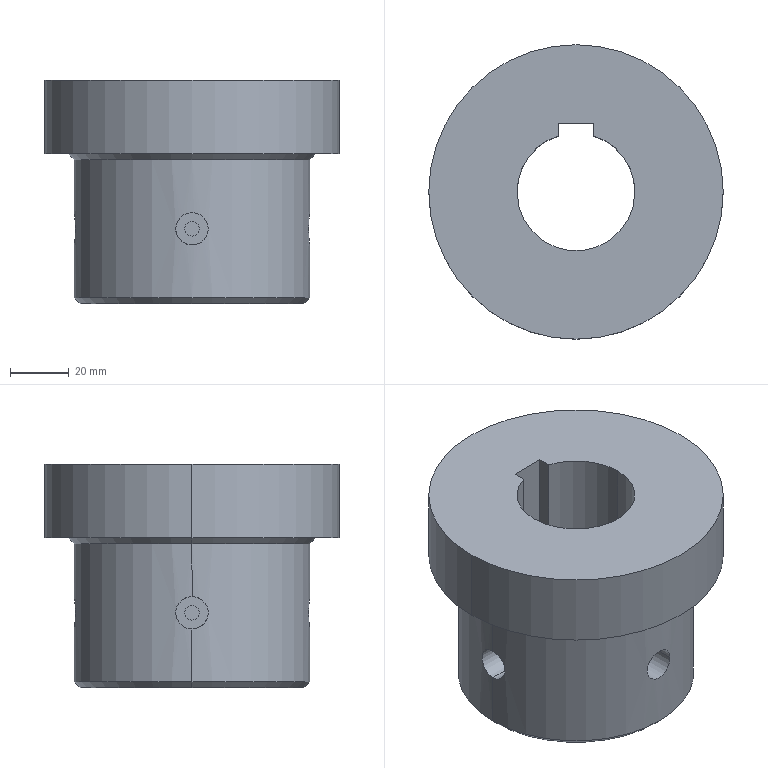Part | SolidWorks | features ICE 3, Chamfer 2, CirPattern 2, HoleWzd 1, RefAxis 1, Revolution 1 | 1 solid | 40 faces | box 100 x 100 x 76 mm | volume 350240 mm3 | cylinder 23 | plane 13 | cone 4 | commonest cylinder face diameters 5 x8 11 x8 40 x3 80 x2 100 x2
STEP:
#1=CARTESIAN_POINT('',(32.,0.,23.));
#2=VERTEX_POINT('',#1);
#3=CARTESIAN_POINT('',(32.,0.,28.));
#4=VERTEX_POINT('',#3);
#5=CARTESIAN_POINT('',(32.,0.,25.5));
#6=DIRECTION('',(-1.,0.,0.));
#7=DIRECTION('',(0.,0.,-1.));
#8=AXIS2_PLACEMENT_3D('',#5,#6,#7);
#9=CIRCLE('',#8,2.5);
#10=EDGE_CURVE('',#2,#4,#9,.T.);
#11=ORIENTED_EDGE('',*,*,#10,.F.);
#12=CARTESIAN_POINT('',(23.3,0.,23.));
#13=VERTEX_POINT('',#12);
#14=CARTESIAN_POINT('',(23.3,0.,23.));
#15=DIRECTION('',(-1.,0.,0.));
#16=VECTOR('',#15,1000.);
#17=LINE('',#14,#16);
#18=EDGE_CURVE('',#2,#13,#17,.T.);
#19=ORIENTED_EDGE('',*,*,#18,.T.);
#20=CARTESIAN_POINT('',(23.3,0.,28.));
#21=VERTEX_POINT('',#20);
#22=CARTESIAN_POINT('',(23.3,0.,25.5));
#23=DIRECTION('',(-1.,0.,0.));
#24=DIRECTION('',(0.,0.,1.));
#25=AXIS2_PLACEMENT_3D('',#22,#23,#24);
#26=CIRCLE('',#25,2.5);
#27=EDGE_CURVE('',#13,#21,#26,.T.);
#28=ORIENTED_EDGE('',*,*,#27,.T.);
#29=CARTESIAN_POINT('',(23.3,0.,28.));
#30=DIRECTION('',(-1.,0.,0.));
#31=VECTOR('',#30,1000.);
#32=LINE('',#29,#31);
#33=EDGE_CURVE('',#4,#21,#32,.T.);
#34=ORIENTED_EDGE('',*,*,#33,.F.);
#35=EDGE_LOOP('',(#11,#19,#28,#34));
#36=FACE_OUTER_BOUND('',#35,.T.);
#37=CARTESIAN_POINT('',(23.3,0.,25.5));
#38=DIRECTION('',(-1.,0.,0.));
#39=DIRECTION('',(0.,0.,1.));
#40=AXIS2_PLACEMENT_3D('',#37,#38,#39);
#41=CYLINDRICAL_SURFACE('',#40,2.5);
#42=ADVANCED_FACE('',(#36),#41,.F.);
#43=CARTESIAN_POINT('',(0.,-32.,23.));
#44=VERTEX_POINT('',#43);
#45=CARTESIAN_POINT('',(0.,-32.,28.));
#46=VERTEX_POINT('',#45);
#47=CARTESIAN_POINT('',(0.,-32.,25.5));
#48=DIRECTION('',(0.,1.,0.));
#49=DIRECTION('',(1.,0.,0.));
#50=AXIS2_PLACEMENT_3D('',#47,#48,#49);
#51=CIRCLE('',#50,2.5);
#52=EDGE_CURVE('',#44,#46,#51,.T.);
#53=ORIENTED_EDGE('',*,*,#52,.F.);
#54=CARTESIAN_POINT('',(0.,-23.3,23.));
#55=VERTEX_POINT('',#54);
#56=CARTESIAN_POINT('',(0.,-23.3,23.));
#57=DIRECTION('',(0.,1.,0.));
#58=VECTOR('',#57,1000.);
#59=LINE('',#56,#58);
#60=EDGE_CURVE('',#44,#55,#59,.T.);
#61=ORIENTED_EDGE('',*,*,#60,.T.);
#62=CARTESIAN_POINT('',(0.,-23.3,28.));
#63=VERTEX_POINT('',#62);
#64=CARTESIAN_POINT('',(0.,-23.3,25.5));
#65=DIRECTION('',(0.,1.,0.));
#66=DIRECTION('',(0.,0.,1.));
#67=AXIS2_PLACEMENT_3D('',#64,#65,#66);
#68=CIRCLE('',#67,2.5);
#69=EDGE_CURVE('',#55,#63,#68,.T.);
#70=ORIENTED_EDGE('',*,*,#69,.T.);
#71=CARTESIAN_POINT('',(0.,-23.3,28.));
#72=DIRECTION('',(0.,1.,0.));
#73=VECTOR('',#72,1000.);
#74=LINE('',#71,#73);
#75=EDGE_CURVE('',#46,#63,#74,.T.);
#76=ORIENTED_EDGE('',*,*,#75,.F.);
#77=EDGE_LOOP('',(#53,#61,#70,#76));
#78=FACE_OUTER_BOUND('',#77,.T.);
#79=CARTESIAN_POINT('',(0.,-23.3,25.5));
#80=DIRECTION('',(0.,1.,0.));
#81=DIRECTION('',(0.,0.,1.));
#82=AXIS2_PLACEMENT_3D('',#79,#80,#81);
#83=CYLINDRICAL_SURFACE('',#82,2.5);
#84=ADVANCED_FACE('',(#78),#83,.F.);
#85=CARTESIAN_POINT('',(5.5,32.,25.5));
#86=VERTEX_POINT('',#85);
#87=CARTESIAN_POINT('',(-5.5,32.,25.5));
#88=VERTEX_POINT('',#87);
#89=CARTESIAN_POINT('',(0.,32.,25.5));
#90=DIRECTION('',(0.,1.,0.));
#91=DIRECTION('',(0.,0.,1.));
#92=AXIS2_PLACEMENT_3D('',#89,#90,#91);
#93=CIRCLE('',#92,5.5);
#94=EDGE_CURVE('',#86,#88,#93,.T.);
#95=ORIENTED_EDGE('',*,*,#94,.F.);
#96=CARTESIAN_POINT('',(5.5,39.62,25.5));
#97=VERTEX_POINT('',#96);
#98=CARTESIAN_POINT('',(5.5,32.,25.5));
#99=DIRECTION('',(0.,1.,0.));
#100=VECTOR('',#99,1000.);
#101=LINE('',#98,#100);
#102=EDGE_CURVE('',#86,#97,#101,.T.);
#103=ORIENTED_EDGE('',*,*,#102,.T.);
#104=CARTESIAN_POINT('',(-5.5,39.62,25.5));
#105=VERTEX_POINT('',#104);
#106=CARTESIAN_POINT('',(-5.5,39.62,25.5));
#107=CARTESIAN_POINT('',(-5.5,39.62,25.136));
#108=CARTESIAN_POINT('',(-5.464,39.625,24.778));
#109=CARTESIAN_POINT('',(-5.359,39.639,24.251));
#110=CARTESIAN_POINT('',(-5.316,39.645,24.076));
#111=CARTESIAN_POINT('',(-5.211,39.659,23.731));
#112=CARTESIAN_POINT('',(-5.149,39.667,23.559));
#113=CARTESIAN_POINT('',(-4.942,39.694,23.059));
#114=CARTESIAN_POINT('',(-4.773,39.715,22.744));
#115=CARTESIAN_POINT('',(-4.374,39.761,22.146));
#116=CARTESIAN_POINT('',(-4.142,39.786,21.863));
#117=CARTESIAN_POINT('',(-3.635,39.835,21.357));
#118=CARTESIAN_POINT('',(-3.358,39.86,21.129));
#119=CARTESIAN_POINT('',(-2.757,39.906,20.727));
#120=CARTESIAN_POINT('',(-2.438,39.927,20.557));
#121=CARTESIAN_POINT('',(-1.941,39.953,20.351));
#122=CARTESIAN_POINT('',(-1.772,39.961,20.29));
#123=CARTESIAN_POINT('',(-1.428,39.975,20.186));
#124=CARTESIAN_POINT('',(-1.251,39.981,20.141));
#125=CARTESIAN_POINT('',(-0.7184,39.995,20.035));
#126=CARTESIAN_POINT('',(-0.3612,40.,20.));
#127=CARTESIAN_POINT('',(0.3572,40.,20.));
#128=CARTESIAN_POINT('',(0.7221,39.995,20.036));
#129=CARTESIAN_POINT('',(1.428,39.976,20.176));
#130=CARTESIAN_POINT('',(1.771,39.962,20.28));
#131=CARTESIAN_POINT('',(2.271,39.936,20.487));
#132=CARTESIAN_POINT('',(2.436,39.926,20.565));
#133=CARTESIAN_POINT('',(2.754,39.905,20.736));
#134=CARTESIAN_POINT('',(2.908,39.894,20.828));
#135=CARTESIAN_POINT('',(3.354,39.86,21.127));
#136=CARTESIAN_POINT('',(3.632,39.836,21.354));
#137=CARTESIAN_POINT('',(4.145,39.785,21.867));
#138=CARTESIAN_POINT('',(4.372,39.761,22.144));
#139=CARTESIAN_POINT('',(4.671,39.726,22.591));
#140=CARTESIAN_POINT('',(4.764,39.715,22.745));
#141=CARTESIAN_POINT('',(4.934,39.695,23.063));
#142=CARTESIAN_POINT('',(5.012,39.685,23.228));
#143=CARTESIAN_POINT('',(5.219,39.658,23.727));
#144=CARTESIAN_POINT('',(5.323,39.644,24.07));
#145=CARTESIAN_POINT('',(5.464,39.625,24.776));
#146=CARTESIAN_POINT('',(5.5,39.62,25.141));
#147=CARTESIAN_POINT('',(5.5,39.62,25.5));
#148=B_SPLINE_CURVE_WITH_KNOTS('',3,(#106,#107,#108,#109,#110,#111,#112,#113,#114,#115,#116,#117,#118,#119,#120,#121,#122,#123,#124,#125,#126,#127,#128,#129,#130,#131,#132,#133,#134,#135,#136,#137,#138,#139,#140,#141,#142,#143,#144,#145,#146,#147),.UNSPECIFIED.,.F.,.F.,(4,2,2,2,2,2,2,2,2,2,2,2,2,2,2,2,2,2,2,2,4),(0.,0.001076,0.001614,0.002152,0.003228,0.004304,0.00538,0.006456,0.006994,0.007532,0.008608,0.009684,0.01076,0.0113,0.01184,0.01291,0.01399,0.01453,0.01506,0.01614,0.01722),.UNSPECIFIED.);
#149=EDGE_CURVE('',#105,#97,#148,.T.);
#150=ORIENTED_EDGE('',*,*,#149,.F.);
#151=CARTESIAN_POINT('',(-5.5,32.,25.5));
#152=DIRECTION('',(0.,1.,0.));
#153=VECTOR('',#152,1000.);
#154=LINE('',#151,#153);
#155=EDGE_CURVE('',#88,#105,#154,.T.);
#156=ORIENTED_EDGE('',*,*,#155,.F.);
#157=EDGE_LOOP('',(#95,#103,#150,#156));
#158=FACE_OUTER_BOUND('',#157,.T.);
#159=CARTESIAN_POINT('',(0.,32.,25.5));
#160=DIRECTION('',(0.,1.,0.));
#161=DIRECTION('',(-1.,0.,0.));
#162=AXIS2_PLACEMENT_3D('',#159,#160,#161);
#163=CYLINDRICAL_SURFACE('',#162,5.5);
#164=ADVANCED_FACE('',(#158),#163,.F.);
#165=CARTESIAN_POINT('',(32.,0.,31.));
#166=VERTEX_POINT('',#165);
#167=CARTESIAN_POINT('',(32.,0.,20.));
#168=VERTEX_POINT('',#167);
#169=CARTESIAN_POINT('',(32.,0.,25.5));
#170=DIRECTION('',(1.,0.,0.));
#171=DIRECTION('',(0.,0.,1.));
#172=AXIS2_PLACEMENT_3D('',#169,#170,#171);
#173=CIRCLE('',#172,5.5);
#174=EDGE_CURVE('',#166,#168,#173,.T.);
#175=ORIENTED_EDGE('',*,*,#174,.F.);
#176=CARTESIAN_POINT('',(40.,0.,31.));
#177=VERTEX_POINT('',#176);
#178=CARTESIAN_POINT('',(32.,0.,31.));
#179=DIRECTION('',(1.,0.,0.));
#180=VECTOR('',#179,1000.);
#181=LINE('',#178,#180);
#182=EDGE_CURVE('',#166,#177,#181,.T.);
#183=ORIENTED_EDGE('',*,*,#182,.T.);
#184=CARTESIAN_POINT('',(40.,0.,20.));
#185=VERTEX_POINT('',#184);
#186=CARTESIAN_POINT('',(40.,0.,20.));
#187=CARTESIAN_POINT('',(40.,-0.3639,20.));
#188=CARTESIAN_POINT('',(39.995,-0.7216,20.036));
#189=CARTESIAN_POINT('',(39.981,-1.249,20.141));
#190=CARTESIAN_POINT('',(39.975,-1.424,20.184));
#191=CARTESIAN_POINT('',(39.961,-1.769,20.289));
#192=CARTESIAN_POINT('',(39.953,-1.941,20.351));
#193=CARTESIAN_POINT('',(39.927,-2.441,20.558));
#194=CARTESIAN_POINT('',(39.906,-2.756,20.727));
#195=CARTESIAN_POINT('',(39.86,-3.354,21.126));
#196=CARTESIAN_POINT('',(39.835,-3.637,21.358));
#197=CARTESIAN_POINT('',(39.786,-4.143,21.865));
#198=CARTESIAN_POINT('',(39.761,-4.371,22.142));
#199=CARTESIAN_POINT('',(39.715,-4.773,22.743));
#200=CARTESIAN_POINT('',(39.694,-4.943,23.063));
#201=CARTESIAN_POINT('',(39.667,-5.149,23.559));
#202=CARTESIAN_POINT('',(39.659,-5.21,23.728));
#203=CARTESIAN_POINT('',(39.645,-5.314,24.072));
#204=CARTESIAN_POINT('',(39.639,-5.359,24.249));
#205=CARTESIAN_POINT('',(39.625,-5.465,24.782));
#206=CARTESIAN_POINT('',(39.62,-5.5,25.139));
#207=CARTESIAN_POINT('',(39.62,-5.5,25.857));
#208=CARTESIAN_POINT('',(39.625,-5.464,26.222));
#209=CARTESIAN_POINT('',(39.644,-5.324,26.928));
#210=CARTESIAN_POINT('',(39.658,-5.22,27.271));
#211=CARTESIAN_POINT('',(39.685,-5.013,27.771));
#212=CARTESIAN_POINT('',(39.695,-4.935,27.936));
#213=CARTESIAN_POINT('',(39.715,-4.764,28.254));
#214=CARTESIAN_POINT('',(39.726,-4.672,28.408));
#215=CARTESIAN_POINT('',(39.761,-4.373,28.854));
#216=CARTESIAN_POINT('',(39.785,-4.146,29.132));
#217=CARTESIAN_POINT('',(39.836,-3.633,29.645));
#218=CARTESIAN_POINT('',(39.86,-3.356,29.872));
#219=CARTESIAN_POINT('',(39.894,-2.909,30.171));
#220=CARTESIAN_POINT('',(39.905,-2.755,30.264));
#221=CARTESIAN_POINT('',(39.926,-2.437,30.434));
#222=CARTESIAN_POINT('',(39.936,-2.272,30.512));
#223=CARTESIAN_POINT('',(39.962,-1.773,30.719));
#224=CARTESIAN_POINT('',(39.976,-1.43,30.823));
#225=CARTESIAN_POINT('',(39.995,-0.724,30.964));
#226=CARTESIAN_POINT('',(40.,-0.3592,31.));
#227=CARTESIAN_POINT('',(40.,0.,31.));
#228=B_SPLINE_CURVE_WITH_KNOTS('',3,(#186,#187,#188,#189,#190,#191,#192,#193,#194,#195,#196,#197,#198,#199,#200,#201,#202,#203,#204,#205,#206,#207,#208,#209,#210,#211,#212,#213,#214,#215,#216,#217,#218,#219,#220,#221,#222,#223,#224,#225,#226,#227),.UNSPECIFIED.,.F.,.F.,(4,2,2,2,2,2,2,2,2,2,2,2,2,2,2,2,2,2,2,2,4),(0.,0.001076,0.001614,0.002152,0.003228,0.004304,0.00538,0.006456,0.006994,0.007532,0.008608,0.009684,0.01076,0.0113,0.01184,0.01291,0.01399,0.01453,0.01506,0.01614,0.01722),.UNSPECIFIED.);
#229=EDGE_CURVE('',#185,#177,#228,.T.);
#230=ORIENTED_EDGE('',*,*,#229,.F.);
#231=CARTESIAN_POINT('',(32.,0.,20.));
#232=DIRECTION('',(1.,0.,0.));
#233=VECTOR('',#232,1000.);
#234=LINE('',#231,#233);
#235=EDGE_CURVE('',#168,#185,#234,.T.);
#236=ORIENTED_EDGE('',*,*,#235,.F.);
#237=EDGE_LOOP('',(#175,#183,#230,#236));
#238=FACE_OUTER_BOUND('',#237,.T.);
#239=CARTESIAN_POINT('',(32.,0.,25.5));
#240=DIRECTION('',(1.,0.,0.));
#241=DIRECTION('',(0.,0.,-1.));
#242=AXIS2_PLACEMENT_3D('',#239,#240,#241);
#243=CYLINDRICAL_SURFACE('',#242,5.5);
#244=ADVANCED_FACE('',(#238),#243,.F.);
#245=CARTESIAN_POINT('',(-5.5,-32.,25.5));
#246=VERTEX_POINT('',#245);
#247=CARTESIAN_POINT('',(5.5,-32.,25.5));
#248=VERTEX_POINT('',#247);
#249=CARTESIAN_POINT('',(0.,-32.,25.5));
#250=DIRECTION('',(0.,-1.,0.));
#251=DIRECTION('',(0.,0.,1.));
#252=AXIS2_PLACEMENT_3D('',#249,#250,#251);
#253=CIRCLE('',#252,5.5);
#254=EDGE_CURVE('',#246,#248,#253,.T.);
#255=ORIENTED_EDGE('',*,*,#254,.F.);
#256=CARTESIAN_POINT('',(-5.5,-39.62,25.5));
#257=VERTEX_POINT('',#256);
#258=CARTESIAN_POINT('',(-5.5,-32.,25.5));
#259=DIRECTION('',(0.,-1.,0.));
#260=VECTOR('',#259,1000.);
#261=LINE('',#258,#260);
#262=EDGE_CURVE('',#246,#257,#261,.T.);
#263=ORIENTED_EDGE('',*,*,#262,.T.);
#264=CARTESIAN_POINT('',(5.5,-39.62,25.5));
#265=VERTEX_POINT('',#264);
#266=CARTESIAN_POINT('',(5.5,-39.62,25.5));
#267=CARTESIAN_POINT('',(5.5,-39.62,25.136));
#268=CARTESIAN_POINT('',(5.464,-39.625,24.778));
#269=CARTESIAN_POINT('',(5.359,-39.639,24.251));
#270=CARTESIAN_POINT('',(5.316,-39.645,24.076));
#271=CARTESIAN_POINT('',(5.211,-39.659,23.731));
#272=CARTESIAN_POINT('',(5.149,-39.667,23.559));
#273=CARTESIAN_POINT('',(4.942,-39.694,23.059));
#274=CARTESIAN_POINT('',(4.773,-39.715,22.744));
#275=CARTESIAN_POINT('',(4.374,-39.761,22.146));
#276=CARTESIAN_POINT('',(4.142,-39.786,21.863));
#277=CARTESIAN_POINT('',(3.635,-39.835,21.357));
#278=CARTESIAN_POINT('',(3.358,-39.86,21.129));
#279=CARTESIAN_POINT('',(2.757,-39.906,20.727));
#280=CARTESIAN_POINT('',(2.438,-39.927,20.557));
#281=CARTESIAN_POINT('',(1.941,-39.953,20.351));
#282=CARTESIAN_POINT('',(1.772,-39.961,20.29));
#283=CARTESIAN_POINT('',(1.428,-39.975,20.186));
#284=CARTESIAN_POINT('',(1.251,-39.981,20.141));
#285=CARTESIAN_POINT('',(0.7184,-39.995,20.035));
#286=CARTESIAN_POINT('',(0.3612,-40.,20.));
#287=CARTESIAN_POINT('',(-0.3572,-40.,20.));
#288=CARTESIAN_POINT('',(-0.7221,-39.995,20.036));
#289=CARTESIAN_POINT('',(-1.428,-39.976,20.176));
#290=CARTESIAN_POINT('',(-1.771,-39.962,20.28));
#291=CARTESIAN_POINT('',(-2.271,-39.936,20.487));
#292=CARTESIAN_POINT('',(-2.436,-39.926,20.565));
#293=CARTESIAN_POINT('',(-2.754,-39.905,20.736));
#294=CARTESIAN_POINT('',(-2.908,-39.894,20.828));
#295=CARTESIAN_POINT('',(-3.354,-39.86,21.127));
#296=CARTESIAN_POINT('',(-3.632,-39.836,21.354));
#297=CARTESIAN_POINT('',(-4.145,-39.785,21.867));
#298=CARTESIAN_POINT('',(-4.372,-39.761,22.144));
#299=CARTESIAN_POINT('',(-4.671,-39.726,22.591));
#300=CARTESIAN_POINT('',(-4.764,-39.715,22.745));
#301=CARTESIAN_POINT('',(-4.934,-39.695,23.063));
#302=CARTESIAN_POINT('',(-5.012,-39.685,23.228));
#303=CARTESIAN_POINT('',(-5.219,-39.658,23.727));
#304=CARTESIAN_POINT('',(-5.323,-39.644,24.07));
#305=CARTESIAN_POINT('',(-5.464,-39.625,24.776));
#306=CARTESIAN_POINT('',(-5.5,-39.62,25.141));
#307=CARTESIAN_POINT('',(-5.5,-39.62,25.5));
#308=B_SPLINE_CURVE_WITH_KNOTS('',3,(#266,#267,#268,#269,#270,#271,#272,#273,#274,#275,#276,#277,#278,#279,#280,#281,#282,#283,#284,#285,#286,#287,#288,#289,#290,#291,#292,#293,#294,#295,#296,#297,#298,#299,#300,#301,#302,#303,#304,#305,#306,#307),.UNSPECIFIED.,.F.,.F.,(4,2,2,2,2,2,2,2,2,2,2,2,2,2,2,2,2,2,2,2,4),(0.,0.001076,0.001614,0.002152,0.003228,0.004304,0.00538,0.006456,0.006994,0.007532,0.008608,0.009684,0.01076,0.0113,0.01184,0.01291,0.01399,0.01453,0.01506,0.01614,0.01722),.UNSPECIFIED.);
#309=EDGE_CURVE('',#265,#257,#308,.T.);
#310=ORIENTED_EDGE('',*,*,#309,.F.);
#311=CARTESIAN_POINT('',(5.5,-32.,25.5));
#312=DIRECTION('',(0.,-1.,0.));
#313=VECTOR('',#312,1000.);
#314=LINE('',#311,#313);
#315=EDGE_CURVE('',#248,#265,#314,.T.);
#316=ORIENTED_EDGE('',*,*,#315,.F.);
#317=EDGE_LOOP('',(#255,#263,#310,#316));
#318=FACE_OUTER_BOUND('',#317,.T.);
#319=CARTESIAN_POINT('',(0.,-32.,25.5));
#320=DIRECTION('',(0.,-1.,0.));
#321=DIRECTION('',(1.,0.,0.));
#322=AXIS2_PLACEMENT_3D('',#319,#320,#321);
#323=CYLINDRICAL_SURFACE('',#322,5.5);
#324=ADVANCED_FACE('',(#318),#323,.F.);
#325=CARTESIAN_POINT('',(-32.,0.,28.));
#326=VERTEX_POINT('',#325);
#327=CARTESIAN_POINT('',(-32.,0.,23.));
#328=VERTEX_POINT('',#327);
#329=CARTESIAN_POINT('',(-32.,0.,25.5));
#330=DIRECTION('',(1.,0.,0.));
#331=DIRECTION('',(0.,0.,1.));
#332=AXIS2_PLACEMENT_3D('',#329,#330,#331);
#333=CIRCLE('',#332,2.5);
#334=EDGE_CURVE('',#326,#328,#333,.T.);
#335=ORIENTED_EDGE('',*,*,#334,.F.);
#336=CARTESIAN_POINT('',(-23.3,0.,28.));
#337=VERTEX_POINT('',#336);
#338=CARTESIAN_POINT('',(-23.3,0.,28.));
#339=DIRECTION('',(1.,0.,0.));
#340=VECTOR('',#339,1000.);
#341=LINE('',#338,#340);
#342=EDGE_CURVE('',#326,#337,#341,.T.);
#343=ORIENTED_EDGE('',*,*,#342,.T.);
#344=CARTESIAN_POINT('',(-23.3,0.,23.));
#345=VERTEX_POINT('',#344);
#346=CARTESIAN_POINT('',(-23.3,0.,25.5));
#347=DIRECTION('',(1.,0.,0.));
#348=DIRECTION('',(0.,0.,-1.));
#349=AXIS2_PLACEMENT_3D('',#346,#347,#348);
#350=CIRCLE('',#349,2.5);
#351=EDGE_CURVE('',#337,#345,#350,.T.);
#352=ORIENTED_EDGE('',*,*,#351,.T.);
#353=CARTESIAN_POINT('',(-23.3,0.,23.));
#354=DIRECTION('',(1.,0.,0.));
#355=VECTOR('',#354,1000.);
#356=LINE('',#353,#355);
#357=EDGE_CURVE('',#328,#345,#356,.T.);
#358=ORIENTED_EDGE('',*,*,#357,.F.);
#359=EDGE_LOOP('',(#335,#343,#352,#358));
#360=FACE_OUTER_BOUND('',#359,.T.);
#361=CARTESIAN_POINT('',(-23.3,0.,25.5));
#362=DIRECTION('',(1.,0.,0.));
#363=DIRECTION('',(0.,0.,-1.));
#364=AXIS2_PLACEMENT_3D('',#361,#362,#363);
#365=CYLINDRICAL_SURFACE('',#364,2.5);
#366=ADVANCED_FACE('',(#360),#365,.F.);
#367=CARTESIAN_POINT('',(-32.,0.,20.));
#368=VERTEX_POINT('',#367);
#369=CARTESIAN_POINT('',(-32.,0.,31.));
#370=VERTEX_POINT('',#369);
#371=CARTESIAN_POINT('',(-32.,0.,25.5));
#372=DIRECTION('',(-1.,0.,0.));
#373=DIRECTION('',(0.,0.,1.));
#374=AXIS2_PLACEMENT_3D('',#371,#372,#373);
#375=CIRCLE('',#374,5.5);
#376=EDGE_CURVE('',#368,#370,#375,.T.);
#377=ORIENTED_EDGE('',*,*,#376,.F.);
#378=CARTESIAN_POINT('',(-40.,0.,20.));
#379=VERTEX_POINT('',#378);
#380=CARTESIAN_POINT('',(-32.,0.,20.));
#381=DIRECTION('',(-1.,0.,0.));
#382=VECTOR('',#381,1000.);
#383=LINE('',#380,#382);
#384=EDGE_CURVE('',#368,#379,#383,.T.);
#385=ORIENTED_EDGE('',*,*,#384,.T.);
#386=CARTESIAN_POINT('',(-40.,0.,31.));
#387=VERTEX_POINT('',#386);
#388=CARTESIAN_POINT('',(-40.,0.,31.));
#389=CARTESIAN_POINT('',(-40.,-0.3639,31.));
#390=CARTESIAN_POINT('',(-39.995,-0.7216,30.964));
#391=CARTESIAN_POINT('',(-39.981,-1.249,30.859));
#392=CARTESIAN_POINT('',(-39.975,-1.424,30.816));
#393=CARTESIAN_POINT('',(-39.961,-1.769,30.711));
#394=CARTESIAN_POINT('',(-39.953,-1.941,30.649));
#395=CARTESIAN_POINT('',(-39.927,-2.441,30.442));
#396=CARTESIAN_POINT('',(-39.906,-2.756,30.273));
#397=CARTESIAN_POINT('',(-39.86,-3.354,29.874));
#398=CARTESIAN_POINT('',(-39.835,-3.637,29.642));
#399=CARTESIAN_POINT('',(-39.786,-4.143,29.135));
#400=CARTESIAN_POINT('',(-39.761,-4.371,28.858));
#401=CARTESIAN_POINT('',(-39.715,-4.773,28.257));
#402=CARTESIAN_POINT('',(-39.694,-4.943,27.937));
#403=CARTESIAN_POINT('',(-39.667,-5.149,27.441));
#404=CARTESIAN_POINT('',(-39.659,-5.21,27.272));
#405=CARTESIAN_POINT('',(-39.645,-5.314,26.928));
#406=CARTESIAN_POINT('',(-39.639,-5.359,26.751));
#407=CARTESIAN_POINT('',(-39.625,-5.465,26.218));
#408=CARTESIAN_POINT('',(-39.62,-5.5,25.861));
#409=CARTESIAN_POINT('',(-39.62,-5.5,25.143));
#410=CARTESIAN_POINT('',(-39.625,-5.464,24.778));
#411=CARTESIAN_POINT('',(-39.644,-5.324,24.072));
#412=CARTESIAN_POINT('',(-39.658,-5.22,23.729));
#413=CARTESIAN_POINT('',(-39.685,-5.013,23.229));
#414=CARTESIAN_POINT('',(-39.695,-4.935,23.064));
#415=CARTESIAN_POINT('',(-39.715,-4.764,22.746));
#416=CARTESIAN_POINT('',(-39.726,-4.672,22.592));
#417=CARTESIAN_POINT('',(-39.761,-4.373,22.146));
#418=CARTESIAN_POINT('',(-39.785,-4.146,21.868));
#419=CARTESIAN_POINT('',(-39.836,-3.633,21.355));
#420=CARTESIAN_POINT('',(-39.86,-3.356,21.128));
#421=CARTESIAN_POINT('',(-39.894,-2.909,20.829));
#422=CARTESIAN_POINT('',(-39.905,-2.755,20.736));
#423=CARTESIAN_POINT('',(-39.926,-2.437,20.566));
#424=CARTESIAN_POINT('',(-39.936,-2.272,20.488));
#425=CARTESIAN_POINT('',(-39.962,-1.773,20.281));
#426=CARTESIAN_POINT('',(-39.976,-1.43,20.177));
#427=CARTESIAN_POINT('',(-39.995,-0.724,20.036));
#428=CARTESIAN_POINT('',(-40.,-0.3592,20.));
#429=CARTESIAN_POINT('',(-40.,0.,20.));
#430=B_SPLINE_CURVE_WITH_KNOTS('',3,(#388,#389,#390,#391,#392,#393,#394,#395,#396,#397,#398,#399,#400,#401,#402,#403,#404,#405,#406,#407,#408,#409,#410,#411,#412,#413,#414,#415,#416,#417,#418,#419,#420,#421,#422,#423,#424,#425,#426,#427,#428,#429),.UNSPECIFIED.,.F.,.F.,(4,2,2,2,2,2,2,2,2,2,2,2,2,2,2,2,2,2,2,2,4),(0.,0.001076,0.001614,0.002152,0.003228,0.004304,0.00538,0.006456,0.006994,0.007532,0.008608,0.009684,0.01076,0.0113,0.01184,0.01291,0.01399,0.01453,0.01506,0.01614,0.01722),.UNSPECIFIED.);
#431=EDGE_CURVE('',#387,#379,#430,.T.);
#432=ORIENTED_EDGE('',*,*,#431,.F.);
#433=CARTESIAN_POINT('',(-32.,0.,31.));
#434=DIRECTION('',(-1.,0.,0.));
#435=VECTOR('',#434,1000.);
#436=LINE('',#433,#435);
#437=EDGE_CURVE('',#370,#387,#436,.T.);
#438=ORIENTED_EDGE('',*,*,#437,.F.);
#439=EDGE_LOOP('',(#377,#385,#432,#438));
#440=FACE_OUTER_BOUND('',#439,.T.);
#441=CARTESIAN_POINT('',(-32.,0.,25.5));
#442=DIRECTION('',(-1.,0.,0.));
#443=DIRECTION('',(0.,0.,1.));
#444=AXIS2_PLACEMENT_3D('',#441,#442,#443);
#445=CYLINDRICAL_SURFACE('',#444,5.5);
#446=ADVANCED_FACE('',(#440),#445,.F.);
#447=CARTESIAN_POINT('',(-20.,0.,0.));
#448=VERTEX_POINT('',#447);
#449=CARTESIAN_POINT('',(20.,0.,0.));
#450=VERTEX_POINT('',#449);
#451=CARTESIAN_POINT('',(0.,0.,0.));
#452=DIRECTION('',(0.,0.,1.));
#453=DIRECTION('',(1.,0.,0.));
#454=AXIS2_PLACEMENT_3D('',#451,#452,#453);
#455=CIRCLE('',#454,20.);
#456=EDGE_CURVE('',#448,#450,#455,.T.);
#457=ORIENTED_EDGE('',*,*,#456,.F.);
#458=CARTESIAN_POINT('',(-20.,0.,76.));
#459=VERTEX_POINT('',#458);
#460=CARTESIAN_POINT('',(-20.,0.,0.));
#461=DIRECTION('',(0.,0.,1.));
#462=VECTOR('',#461,1000.);
#463=LINE('',#460,#462);
#464=EDGE_CURVE('',#448,#459,#463,.T.);
#465=ORIENTED_EDGE('',*,*,#464,.T.);
#466=CARTESIAN_POINT('',(20.,0.,76.));
#467=VERTEX_POINT('',#466);
#468=CARTESIAN_POINT('',(0.,0.,76.));
#469=DIRECTION('',(0.,0.,1.));
#470=DIRECTION('',(1.,0.,0.));
#471=AXIS2_PLACEMENT_3D('',#468,#469,#470);
#472=CIRCLE('',#471,20.);
#473=EDGE_CURVE('',#459,#467,#472,.T.);
#474=ORIENTED_EDGE('',*,*,#473,.T.);
#475=CARTESIAN_POINT('',(20.,0.,0.));
#476=DIRECTION('',(0.,0.,1.));
#477=VECTOR('',#476,1000.);
#478=LINE('',#475,#477);
#479=EDGE_CURVE('',#450,#467,#478,.T.);
#480=ORIENTED_EDGE('',*,*,#479,.F.);
#481=EDGE_LOOP('',(#457,#465,#474,#480));
#482=FACE_OUTER_BOUND('',#481,.T.);
#483=CARTESIAN_POINT('',(0.,0.,0.));
#484=DIRECTION('',(0.,0.,1.));
#485=DIRECTION('',(1.,0.,0.));
#486=AXIS2_PLACEMENT_3D('',#483,#484,#485);
#487=CYLINDRICAL_SURFACE('',#486,20.);
#488=ADVANCED_FACE('',(#482),#487,.F.);
#489=CARTESIAN_POINT('',(6.,19.079,0.));
#490=VERTEX_POINT('',#489);
#491=CARTESIAN_POINT('',(0.,0.,0.));
#492=DIRECTION('',(0.,0.,1.));
#493=DIRECTION('',(1.,0.,0.));
#494=AXIS2_PLACEMENT_3D('',#491,#492,#493);
#495=CIRCLE('',#494,20.);
#496=EDGE_CURVE('',#450,#490,#495,.T.);
#497=ORIENTED_EDGE('',*,*,#496,.F.);
#498=ORIENTED_EDGE('',*,*,#479,.T.);
#499=CARTESIAN_POINT('',(6.,19.079,76.));
#500=VERTEX_POINT('',#499);
#501=CARTESIAN_POINT('',(0.,0.,76.));
#502=DIRECTION('',(0.,0.,1.));
#503=DIRECTION('',(1.,0.,0.));
#504=AXIS2_PLACEMENT_3D('',#501,#502,#503);
#505=CIRCLE('',#504,20.);
#506=EDGE_CURVE('',#467,#500,#505,.T.);
#507=ORIENTED_EDGE('',*,*,#506,.T.);
#508=CARTESIAN_POINT('',(6.,19.079,76.));
#509=DIRECTION('',(0.,0.,-1.));
#510=VECTOR('',#509,1000.);
#511=LINE('',#508,#510);
#512=EDGE_CURVE('',#500,#490,#511,.T.);
#513=ORIENTED_EDGE('',*,*,#512,.T.);
#514=EDGE_LOOP('',(#497,#498,#507,#513));
#515=FACE_OUTER_BOUND('',#514,.T.);
#516=CARTESIAN_POINT('',(0.,0.,0.));
#517=DIRECTION('',(0.,0.,1.));
#518=DIRECTION('',(1.,0.,0.));
#519=AXIS2_PLACEMENT_3D('',#516,#517,#518);
#520=CYLINDRICAL_SURFACE('',#519,20.);
#521=ADVANCED_FACE('',(#515),#520,.F.);
#522=CARTESIAN_POINT('',(-38.,0.,0.));
#523=VERTEX_POINT('',#522);
#524=CARTESIAN_POINT('',(38.,0.,0.));
#525=VERTEX_POINT('',#524);
#526=CARTESIAN_POINT('',(0.,0.,0.));
#527=DIRECTION('',(0.,0.,-1.));
#528=DIRECTION('',(1.,0.,0.));
#529=AXIS2_PLACEMENT_3D('',#526,#527,#528);
#530=CIRCLE('',#529,38.);
#531=EDGE_CURVE('',#523,#525,#530,.T.);
#532=ORIENTED_EDGE('',*,*,#531,.F.);
#533=CARTESIAN_POINT('',(-40.,0.,2.));
#534=VERTEX_POINT('',#533);
#535=CARTESIAN_POINT('',(-40.,0.,2.));
#536=DIRECTION('',(-0.7071,0.,0.7071));
#537=VECTOR('',#536,1000.);
#538=LINE('',#535,#537);
#539=EDGE_CURVE('',#523,#534,#538,.T.);
#540=ORIENTED_EDGE('',*,*,#539,.T.);
#541=CARTESIAN_POINT('',(40.,0.,2.));
#542=VERTEX_POINT('',#541);
#543=CARTESIAN_POINT('',(0.,0.,2.));
#544=DIRECTION('',(0.,0.,1.));
#545=DIRECTION('',(1.,0.,0.));
#546=AXIS2_PLACEMENT_3D('',#543,#544,#545);
#547=CIRCLE('',#546,40.);
#548=EDGE_CURVE('',#542,#534,#547,.T.);
#549=ORIENTED_EDGE('',*,*,#548,.F.);
#550=CARTESIAN_POINT('',(40.,0.,2.));
#551=DIRECTION('',(0.7071,0.,0.7071));
#552=VECTOR('',#551,1000.);
#553=LINE('',#550,#552);
#554=EDGE_CURVE('',#525,#542,#553,.T.);
#555=ORIENTED_EDGE('',*,*,#554,.F.);
#556=EDGE_LOOP('',(#532,#540,#549,#555));
#557=FACE_OUTER_BOUND('',#556,.T.);
#558=CARTESIAN_POINT('',(0.,0.,2.));
#559=DIRECTION('',(0.,0.,1.));
#560=DIRECTION('',(1.,0.,0.));
#561=AXIS2_PLACEMENT_3D('',#558,#559,#560);
#562=CONICAL_SURFACE('',#561,40.,0.7854);
#563=ADVANCED_FACE('',(#557),#562,.T.);
#564=CARTESIAN_POINT('',(-40.,0.,49.));
#565=VERTEX_POINT('',#564);
#566=CARTESIAN_POINT('',(40.,0.,49.));
#567=VERTEX_POINT('',#566);
#568=CARTESIAN_POINT('',(0.,0.,49.));
#569=DIRECTION('',(0.,0.,-1.));
#570=DIRECTION('',(1.,0.,0.));
#571=AXIS2_PLACEMENT_3D('',#568,#569,#570);
#572=CIRCLE('',#571,40.);
#573=EDGE_CURVE('',#565,#567,#572,.T.);
#574=ORIENTED_EDGE('',*,*,#573,.F.);
#575=CARTESIAN_POINT('',(-42.,0.,51.));
#576=VERTEX_POINT('',#575);
#577=CARTESIAN_POINT('',(-42.,0.,51.));
#578=DIRECTION('',(-0.7071,0.,0.7071));
#579=VECTOR('',#578,1000.);
#580=LINE('',#577,#579);
#581=EDGE_CURVE('',#565,#576,#580,.T.);
#582=ORIENTED_EDGE('',*,*,#581,.T.);
#583=CARTESIAN_POINT('',(42.,0.,51.));
#584=VERTEX_POINT('',#583);
#585=CARTESIAN_POINT('',(0.,0.,51.));
#586=DIRECTION('',(0.,0.,1.));
#587=DIRECTION('',(1.,0.,0.));
#588=AXIS2_PLACEMENT_3D('',#585,#586,#587);
#589=CIRCLE('',#588,42.);
#590=EDGE_CURVE('',#584,#576,#589,.T.);
#591=ORIENTED_EDGE('',*,*,#590,.F.);
#592=CARTESIAN_POINT('',(42.,0.,51.));
#593=DIRECTION('',(0.7071,0.,0.7071));
#594=VECTOR('',#593,1000.);
#595=LINE('',#592,#594);
#596=EDGE_CURVE('',#567,#584,#595,.T.);
#597=ORIENTED_EDGE('',*,*,#596,.F.);
#598=EDGE_LOOP('',(#574,#582,#591,#597));
#599=FACE_OUTER_BOUND('',#598,.T.);
#600=CARTESIAN_POINT('',(0.,0.,51.));
#601=DIRECTION('',(0.,0.,1.));
#602=DIRECTION('',(1.,0.,0.));
#603=AXIS2_PLACEMENT_3D('',#600,#601,#602);
#604=CONICAL_SURFACE('',#603,42.,0.7854);
#605=ADVANCED_FACE('',(#599),#604,.T.);
#606=CARTESIAN_POINT('',(50.,0.,51.));
#607=VERTEX_POINT('',#606);
#608=CARTESIAN_POINT('',(-50.,0.,51.));
#609=VERTEX_POINT('',#608);
#610=CARTESIAN_POINT('',(0.,0.,51.));
#611=DIRECTION('',(0.,0.,1.));
#612=DIRECTION('',(1.,0.,0.));
#613=AXIS2_PLACEMENT_3D('',#610,#611,#612);
#614=CIRCLE('',#613,50.);
#615=EDGE_CURVE('',#607,#609,#614,.T.);
#616=ORIENTED_EDGE('',*,*,#615,.T.);
#617=CARTESIAN_POINT('',(-50.,0.,76.));
#618=VERTEX_POINT('',#617);
#619=CARTESIAN_POINT('',(-50.,0.,0.));
#620=DIRECTION('',(0.,0.,1.));
#621=VECTOR('',#620,1000.);
#622=LINE('',#619,#621);
#623=EDGE_CURVE('',#609,#618,#622,.T.);
#624=ORIENTED_EDGE('',*,*,#623,.T.);
#625=CARTESIAN_POINT('',(50.,0.,76.));
#626=VERTEX_POINT('',#625);
#627=CARTESIAN_POINT('',(0.,0.,76.));
#628=DIRECTION('',(0.,0.,1.));
#629=DIRECTION('',(1.,0.,0.));
#630=AXIS2_PLACEMENT_3D('',#627,#628,#629);
#631=CIRCLE('',#630,50.);
#632=EDGE_CURVE('',#626,#618,#631,.T.);
#633=ORIENTED_EDGE('',*,*,#632,.F.);
#634=CARTESIAN_POINT('',(50.,0.,0.));
#635=DIRECTION('',(0.,0.,1.));
#636=VECTOR('',#635,1000.);
#637=LINE('',#634,#636);
#638=EDGE_CURVE('',#607,#626,#637,.T.);
#639=ORIENTED_EDGE('',*,*,#638,.F.);
#640=EDGE_LOOP('',(#616,#624,#633,#639));
#641=FACE_OUTER_BOUND('',#640,.T.);
#642=CARTESIAN_POINT('',(0.,0.,0.));
#643=DIRECTION('',(0.,0.,1.));
#644=DIRECTION('',(1.,0.,0.));
#645=AXIS2_PLACEMENT_3D('',#642,#643,#644);
#646=CYLINDRICAL_SURFACE('',#645,50.);
#647=ADVANCED_FACE('',(#641),#646,.T.);
#648=ORIENTED_EDGE('',*,*,#149,.T.);
#649=CARTESIAN_POINT('',(5.5,39.62,25.5));
#650=CARTESIAN_POINT('',(5.5,39.62,25.859));
#651=CARTESIAN_POINT('',(5.465,39.625,26.216));
#652=CARTESIAN_POINT('',(5.324,39.644,26.927));
#653=CARTESIAN_POINT('',(5.219,39.658,27.274));
#654=CARTESIAN_POINT('',(5.013,39.685,27.77));
#655=CARTESIAN_POINT('',(4.936,39.694,27.932));
#656=CARTESIAN_POINT('',(4.767,39.715,28.25));
#657=CARTESIAN_POINT('',(4.673,39.726,28.406));
#658=CARTESIAN_POINT('',(4.372,39.761,28.856));
#659=CARTESIAN_POINT('',(4.145,39.785,29.133));
#660=CARTESIAN_POINT('',(3.638,39.835,29.64));
#661=CARTESIAN_POINT('',(3.356,39.86,29.872));
#662=CARTESIAN_POINT('',(2.759,39.906,30.271));
#663=CARTESIAN_POINT('',(2.444,39.927,30.441));
#664=CARTESIAN_POINT('',(1.944,39.953,30.648));
#665=CARTESIAN_POINT('',(1.772,39.961,30.71));
#666=CARTESIAN_POINT('',(1.427,39.975,30.815));
#667=CARTESIAN_POINT('',(1.253,39.981,30.858));
#668=CARTESIAN_POINT('',(0.7254,39.995,30.964));
#669=CARTESIAN_POINT('',(0.3673,40.,31.));
#670=CARTESIAN_POINT('',(-0.3598,40.,31.));
#671=CARTESIAN_POINT('',(-0.7174,39.995,30.965));
#672=CARTESIAN_POINT('',(-1.245,39.981,30.86));
#673=CARTESIAN_POINT('',(-1.42,39.975,30.817));
#674=CARTESIAN_POINT('',(-1.766,39.961,30.712));
#675=CARTESIAN_POINT('',(-1.937,39.953,30.651));
#676=CARTESIAN_POINT('',(-2.437,39.927,30.444));
#677=CARTESIAN_POINT('',(-2.752,39.906,30.275));
#678=CARTESIAN_POINT('',(-3.35,39.861,29.877));
#679=CARTESIAN_POINT('',(-3.633,39.835,29.645));
#680=CARTESIAN_POINT('',(-4.14,39.786,29.139));
#681=CARTESIAN_POINT('',(-4.368,39.761,28.862));
#682=CARTESIAN_POINT('',(-4.77,39.715,28.261));
#683=CARTESIAN_POINT('',(-4.941,39.694,27.942));
#684=CARTESIAN_POINT('',(-5.216,39.659,27.281));
#685=CARTESIAN_POINT('',(-5.322,39.644,26.934));
#686=CARTESIAN_POINT('',(-5.464,39.625,26.223));
#687=CARTESIAN_POINT('',(-5.5,39.62,25.864));
#688=CARTESIAN_POINT('',(-5.5,39.62,25.5));
#689=B_SPLINE_CURVE_WITH_KNOTS('',3,(#649,#650,#651,#652,#653,#654,#655,#656,#657,#658,#659,#660,#661,#662,#663,#664,#665,#666,#667,#668,#669,#670,#671,#672,#673,#674,#675,#676,#677,#678,#679,#680,#681,#682,#683,#684,#685,#686,#687,#688),.UNSPECIFIED.,.F.,.F.,(4,2,2,2,2,2,2,2,2,2,2,2,2,2,2,2,2,2,2,4),(0.01722,0.01829,0.01937,0.01991,0.02044,0.02152,0.02259,0.02367,0.02421,0.02475,0.02582,0.0269,0.02744,0.02797,0.02905,0.03012,0.0312,0.03228,0.03335,0.03443),.UNSPECIFIED.);
#690=EDGE_CURVE('',#97,#105,#689,.T.);
#691=ORIENTED_EDGE('',*,*,#690,.T.);
#692=EDGE_LOOP('',(#648,#691));
#693=FACE_BOUND('',#692,.T.);
#694=ORIENTED_EDGE('',*,*,#548,.T.);
#695=CARTESIAN_POINT('',(-40.,0.,0.));
#696=DIRECTION('',(0.,0.,1.));
#697=VECTOR('',#696,1000.);
#698=LINE('',#695,#697);
#699=EDGE_CURVE('',#534,#379,#698,.T.);
#700=ORIENTED_EDGE('',*,*,#699,.T.);
#701=CARTESIAN_POINT('',(-40.,0.,20.));
#702=CARTESIAN_POINT('',(-40.,0.3591,20.));
#703=CARTESIAN_POINT('',(-39.995,0.7163,20.035));
#704=CARTESIAN_POINT('',(-39.976,1.427,20.176));
#705=CARTESIAN_POINT('',(-39.962,1.774,20.281));
#706=CARTESIAN_POINT('',(-39.936,2.27,20.487));
#707=CARTESIAN_POINT('',(-39.926,2.432,20.564));
#708=CARTESIAN_POINT('',(-39.906,2.75,20.733));
#709=CARTESIAN_POINT('',(-39.895,2.906,20.827));
#710=CARTESIAN_POINT('',(-39.86,3.356,21.128));
#711=CARTESIAN_POINT('',(-39.836,3.633,21.355));
#712=CARTESIAN_POINT('',(-39.786,4.14,21.862));
#713=CARTESIAN_POINT('',(-39.761,4.372,22.144));
#714=CARTESIAN_POINT('',(-39.715,4.771,22.741));
#715=CARTESIAN_POINT('',(-39.694,4.941,23.056));
#716=CARTESIAN_POINT('',(-39.667,5.148,23.556));
#717=CARTESIAN_POINT('',(-39.659,5.21,23.728));
#718=CARTESIAN_POINT('',(-39.645,5.315,24.073));
#719=CARTESIAN_POINT('',(-39.639,5.358,24.247));
#720=CARTESIAN_POINT('',(-39.625,5.464,24.775));
#721=CARTESIAN_POINT('',(-39.62,5.5,25.133));
#722=CARTESIAN_POINT('',(-39.62,5.5,25.86));
#723=CARTESIAN_POINT('',(-39.625,5.465,26.217));
#724=CARTESIAN_POINT('',(-39.639,5.36,26.745));
#725=CARTESIAN_POINT('',(-39.645,5.317,26.92));
#726=CARTESIAN_POINT('',(-39.659,5.212,27.266));
#727=CARTESIAN_POINT('',(-39.667,5.151,27.437));
#728=CARTESIAN_POINT('',(-39.694,4.944,27.936));
#729=CARTESIAN_POINT('',(-39.714,4.775,28.252));
#730=CARTESIAN_POINT('',(-39.76,4.377,28.85));
#731=CARTESIAN_POINT('',(-39.785,4.145,29.133));
#732=CARTESIAN_POINT('',(-39.835,3.639,29.64));
#733=CARTESIAN_POINT('',(-39.86,3.362,29.868));
#734=CARTESIAN_POINT('',(-39.906,2.761,30.27));
#735=CARTESIAN_POINT('',(-39.927,2.442,30.441));
#736=CARTESIAN_POINT('',(-39.962,1.781,30.716));
#737=CARTESIAN_POINT('',(-39.976,1.434,30.822));
#738=CARTESIAN_POINT('',(-39.995,0.7233,30.964));
#739=CARTESIAN_POINT('',(-40.,0.3638,31.));
#740=CARTESIAN_POINT('',(-40.,0.,31.));
#741=B_SPLINE_CURVE_WITH_KNOTS('',3,(#701,#702,#703,#704,#705,#706,#707,#708,#709,#710,#711,#712,#713,#714,#715,#716,#717,#718,#719,#720,#721,#722,#723,#724,#725,#726,#727,#728,#729,#730,#731,#732,#733,#734,#735,#736,#737,#738,#739,#740),.UNSPECIFIED.,.F.,.F.,(4,2,2,2,2,2,2,2,2,2,2,2,2,2,2,2,2,2,2,4),(0.01722,0.01829,0.01937,0.01991,0.02044,0.02152,0.02259,0.02367,0.02421,0.02475,0.02582,0.0269,0.02744,0.02797,0.02905,0.03012,0.0312,0.03228,0.03335,0.03443),.UNSPECIFIED.);
#742=EDGE_CURVE('',#379,#387,#741,.T.);
#743=ORIENTED_EDGE('',*,*,#742,.T.);
#744=CARTESIAN_POINT('',(-40.,0.,0.));
#745=DIRECTION('',(0.,0.,1.));
#746=VECTOR('',#745,1000.);
#747=LINE('',#744,#746);
#748=EDGE_CURVE('',#387,#565,#747,.T.);
#749=ORIENTED_EDGE('',*,*,#748,.T.);
#750=ORIENTED_EDGE('',*,*,#573,.T.);
#751=CARTESIAN_POINT('',(40.,0.,0.));
#752=DIRECTION('',(0.,0.,1.));
#753=VECTOR('',#752,1000.);
#754=LINE('',#751,#753);
#755=EDGE_CURVE('',#177,#567,#754,.T.);
#756=ORIENTED_EDGE('',*,*,#755,.F.);
#757=CARTESIAN_POINT('',(40.,0.,31.));
#758=CARTESIAN_POINT('',(40.,0.3591,31.));
#759=CARTESIAN_POINT('',(39.995,0.7163,30.965));
#760=CARTESIAN_POINT('',(39.976,1.427,30.824));
#761=CARTESIAN_POINT('',(39.962,1.774,30.719));
#762=CARTESIAN_POINT('',(39.936,2.27,30.513));
#763=CARTESIAN_POINT('',(39.926,2.432,30.436));
#764=CARTESIAN_POINT('',(39.906,2.75,30.267));
#765=CARTESIAN_POINT('',(39.895,2.906,30.173));
#766=CARTESIAN_POINT('',(39.86,3.356,29.872));
#767=CARTESIAN_POINT('',(39.836,3.633,29.645));
#768=CARTESIAN_POINT('',(39.786,4.14,29.138));
#769=CARTESIAN_POINT('',(39.761,4.372,28.856));
#770=CARTESIAN_POINT('',(39.715,4.771,28.259));
#771=CARTESIAN_POINT('',(39.694,4.941,27.944));
#772=CARTESIAN_POINT('',(39.667,5.148,27.444));
#773=CARTESIAN_POINT('',(39.659,5.21,27.272));
#774=CARTESIAN_POINT('',(39.645,5.315,26.927));
#775=CARTESIAN_POINT('',(39.639,5.358,26.753));
#776=CARTESIAN_POINT('',(39.625,5.464,26.225));
#777=CARTESIAN_POINT('',(39.62,5.5,25.867));
#778=CARTESIAN_POINT('',(39.62,5.5,25.14));
#779=CARTESIAN_POINT('',(39.625,5.465,24.783));
#780=CARTESIAN_POINT('',(39.639,5.36,24.255));
#781=CARTESIAN_POINT('',(39.645,5.317,24.08));
#782=CARTESIAN_POINT('',(39.659,5.212,23.734));
#783=CARTESIAN_POINT('',(39.667,5.151,23.563));
#784=CARTESIAN_POINT('',(39.694,4.944,23.064));
#785=CARTESIAN_POINT('',(39.714,4.775,22.748));
#786=CARTESIAN_POINT('',(39.76,4.377,22.15));
#787=CARTESIAN_POINT('',(39.785,4.145,21.867));
#788=CARTESIAN_POINT('',(39.835,3.639,21.36));
#789=CARTESIAN_POINT('',(39.86,3.362,21.132));
#790=CARTESIAN_POINT('',(39.906,2.761,20.73));
#791=CARTESIAN_POINT('',(39.927,2.442,20.559));
#792=CARTESIAN_POINT('',(39.962,1.781,20.284));
#793=CARTESIAN_POINT('',(39.976,1.434,20.178));
#794=CARTESIAN_POINT('',(39.995,0.7233,20.036));
#795=CARTESIAN_POINT('',(40.,0.3638,20.));
#796=CARTESIAN_POINT('',(40.,0.,20.));
#797=B_SPLINE_CURVE_WITH_KNOTS('',3,(#757,#758,#759,#760,#761,#762,#763,#764,#765,#766,#767,#768,#769,#770,#771,#772,#773,#774,#775,#776,#777,#778,#779,#780,#781,#782,#783,#784,#785,#786,#787,#788,#789,#790,#791,#792,#793,#794,#795,#796),.UNSPECIFIED.,.F.,.F.,(4,2,2,2,2,2,2,2,2,2,2,2,2,2,2,2,2,2,2,4),(0.01722,0.01829,0.01937,0.01991,0.02044,0.02152,0.02259,0.02367,0.02421,0.02475,0.02582,0.0269,0.02744,0.02797,0.02905,0.03012,0.0312,0.03228,0.03335,0.03443),.UNSPECIFIED.);
#798=EDGE_CURVE('',#177,#185,#797,.T.);
#799=ORIENTED_EDGE('',*,*,#798,.T.);
#800=CARTESIAN_POINT('',(40.,0.,0.));
#801=DIRECTION('',(0.,0.,1.));
#802=VECTOR('',#801,1000.);
#803=LINE('',#800,#802);
#804=EDGE_CURVE('',#542,#185,#803,.T.);
#805=ORIENTED_EDGE('',*,*,#804,.F.);
#806=EDGE_LOOP('',(#694,#700,#743,#749,#750,#756,#799,#805));
#807=FACE_OUTER_BOUND('',#806,.T.);
#808=CARTESIAN_POINT('',(0.,0.,0.));
#809=DIRECTION('',(0.,0.,1.));
#810=DIRECTION('',(1.,0.,0.));
#811=AXIS2_PLACEMENT_3D('',#808,#809,#810);
#812=CYLINDRICAL_SURFACE('',#811,40.);
#813=ADVANCED_FACE('',(#693,#807),#812,.T.);
#814=CARTESIAN_POINT('',(0.,32.,28.));
#815=VERTEX_POINT('',#814);
#816=CARTESIAN_POINT('',(0.,32.,23.));
#817=VERTEX_POINT('',#816);
#818=CARTESIAN_POINT('',(0.,32.,25.5));
#819=DIRECTION('',(0.,-1.,0.));
#820=DIRECTION('',(-1.,0.,0.));
#821=AXIS2_PLACEMENT_3D('',#818,#819,#820);
#822=CIRCLE('',#821,2.5);
#823=EDGE_CURVE('',#815,#817,#822,.T.);
#824=ORIENTED_EDGE('',*,*,#823,.F.);
#825=CARTESIAN_POINT('',(0.,23.3,28.));
#826=VERTEX_POINT('',#825);
#827=CARTESIAN_POINT('',(0.,23.3,28.));
#828=DIRECTION('',(0.,-1.,0.));
#829=VECTOR('',#828,1000.);
#830=LINE('',#827,#829);
#831=EDGE_CURVE('',#815,#826,#830,.T.);
#832=ORIENTED_EDGE('',*,*,#831,.T.);
#833=CARTESIAN_POINT('',(0.,23.3,23.));
#834=VERTEX_POINT('',#833);
#835=CARTESIAN_POINT('',(0.,23.3,25.5));
#836=DIRECTION('',(0.,-1.,0.));
#837=DIRECTION('',(0.,0.,-1.));
#838=AXIS2_PLACEMENT_3D('',#835,#836,#837);
#839=CIRCLE('',#838,2.5);
#840=EDGE_CURVE('',#826,#834,#839,.T.);
#841=ORIENTED_EDGE('',*,*,#840,.T.);
#842=CARTESIAN_POINT('',(0.,23.3,23.));
#843=DIRECTION('',(0.,-1.,0.));
#844=VECTOR('',#843,1000.);
#845=LINE('',#842,#844);
#846=EDGE_CURVE('',#817,#834,#845,.T.);
#847=ORIENTED_EDGE('',*,*,#846,.F.);
#848=EDGE_LOOP('',(#824,#832,#841,#847));
#849=FACE_OUTER_BOUND('',#848,.T.);
#850=CARTESIAN_POINT('',(0.,23.3,25.5));
#851=DIRECTION('',(0.,-1.,0.));
#852=DIRECTION('',(0.,0.,-1.));
#853=AXIS2_PLACEMENT_3D('',#850,#851,#852);
#854=CYLINDRICAL_SURFACE('',#853,2.5);
#855=ADVANCED_FACE('',(#849),#854,.F.);
#856=ORIENTED_EDGE('',*,*,#831,.F.);
#857=CARTESIAN_POINT('',(0.,32.,25.5));
#858=DIRECTION('',(0.,-1.,0.));
#859=DIRECTION('',(-1.,0.,0.));
#860=AXIS2_PLACEMENT_3D('',#857,#858,#859);
#861=CIRCLE('',#860,2.5);
#862=EDGE_CURVE('',#817,#815,#861,.T.);
#863=ORIENTED_EDGE('',*,*,#862,.F.);
#864=ORIENTED_EDGE('',*,*,#846,.T.);
#865=CARTESIAN_POINT('',(0.,23.3,25.5));
#866=DIRECTION('',(0.,-1.,0.));
#867=DIRECTION('',(0.,0.,-1.));
#868=AXIS2_PLACEMENT_3D('',#865,#866,#867);
#869=CIRCLE('',#868,2.5);
#870=EDGE_CURVE('',#834,#826,#869,.T.);
#871=ORIENTED_EDGE('',*,*,#870,.T.);
#872=EDGE_LOOP('',(#856,#863,#864,#871));
#873=FACE_OUTER_BOUND('',#872,.T.);
#874=CARTESIAN_POINT('',(0.,23.3,25.5));
#875=DIRECTION('',(0.,-1.,0.));
#876=DIRECTION('',(0.,0.,-1.));
#877=AXIS2_PLACEMENT_3D('',#874,#875,#876);
#878=CYLINDRICAL_SURFACE('',#877,2.5);
#879=ADVANCED_FACE('',(#873),#878,.F.);
#880=CARTESIAN_POINT('',(0.,0.,0.));
#881=DIRECTION('',(0.,0.,-1.));
#882=DIRECTION('',(1.,0.,0.));
#883=AXIS2_PLACEMENT_3D('',#880,#881,#882);
#884=CIRCLE('',#883,38.);
#885=EDGE_CURVE('',#525,#523,#884,.T.);
#886=ORIENTED_EDGE('',*,*,#885,.T.);
#887=ORIENTED_EDGE('',*,*,#531,.T.);
#888=EDGE_LOOP('',(#886,#887));
#889=FACE_OUTER_BOUND('',#888,.T.);
#890=CARTESIAN_POINT('',(-6.,19.079,0.));
#891=VERTEX_POINT('',#890);
#892=CARTESIAN_POINT('',(0.,0.,0.));
#893=DIRECTION('',(0.,0.,1.));
#894=DIRECTION('',(1.,0.,0.));
#895=AXIS2_PLACEMENT_3D('',#892,#893,#894);
#896=CIRCLE('',#895,20.);
#897=EDGE_CURVE('',#891,#448,#896,.T.);
#898=ORIENTED_EDGE('',*,*,#897,.T.);
#899=ORIENTED_EDGE('',*,*,#456,.T.);
#900=ORIENTED_EDGE('',*,*,#496,.T.);
#901=CARTESIAN_POINT('',(6.,23.3,0.));
#902=VERTEX_POINT('',#901);
#903=CARTESIAN_POINT('',(6.,19.079,0.));
#904=DIRECTION('',(0.,-1.,0.));
#905=VECTOR('',#904,1000.);
#906=LINE('',#903,#905);
#907=EDGE_CURVE('',#902,#490,#906,.T.);
#908=ORIENTED_EDGE('',*,*,#907,.F.);
#909=CARTESIAN_POINT('',(-6.,23.3,0.));
#910=VERTEX_POINT('',#909);
#911=CARTESIAN_POINT('',(6.,23.3,0.));
#912=DIRECTION('',(1.,0.,0.));
#913=VECTOR('',#912,1000.);
#914=LINE('',#911,#913);
#915=EDGE_CURVE('',#910,#902,#914,.T.);
#916=ORIENTED_EDGE('',*,*,#915,.F.);
#917=CARTESIAN_POINT('',(-6.,19.079,0.));
#918=DIRECTION('',(0.,1.,0.));
#919=VECTOR('',#918,1000.);
#920=LINE('',#917,#919);
#921=EDGE_CURVE('',#891,#910,#920,.T.);
#922=ORIENTED_EDGE('',*,*,#921,.F.);
#923=EDGE_LOOP('',(#898,#899,#900,#908,#916,#922));
#924=FACE_BOUND('',#923,.T.);
#925=CARTESIAN_POINT('',(0.,21.,0.));
#926=DIRECTION('',(0.,0.,1.));
#927=DIRECTION('',(1.,0.,0.));
#928=AXIS2_PLACEMENT_3D('',#925,#926,#927);
#929=PLANE('',#928);
#930=ADVANCED_FACE('',(#889,#924),#929,.F.);
#931=ORIENTED_EDGE('',*,*,#699,.F.);
#932=CARTESIAN_POINT('',(0.,0.,2.));
#933=DIRECTION('',(0.,0.,1.));
#934=DIRECTION('',(1.,0.,0.));
#935=AXIS2_PLACEMENT_3D('',#932,#933,#934);
#936=CIRCLE('',#935,40.);
#937=EDGE_CURVE('',#534,#542,#936,.T.);
#938=ORIENTED_EDGE('',*,*,#937,.T.);
#939=ORIENTED_EDGE('',*,*,#804,.T.);
#940=ORIENTED_EDGE('',*,*,#229,.T.);
#941=ORIENTED_EDGE('',*,*,#755,.T.);
#942=CARTESIAN_POINT('',(0.,0.,49.));
#943=DIRECTION('',(0.,0.,-1.));
#944=DIRECTION('',(1.,0.,0.));
#945=AXIS2_PLACEMENT_3D('',#942,#943,#944);
#946=CIRCLE('',#945,40.);
#947=EDGE_CURVE('',#567,#565,#946,.T.);
#948=ORIENTED_EDGE('',*,*,#947,.T.);
#949=ORIENTED_EDGE('',*,*,#748,.F.);
#950=ORIENTED_EDGE('',*,*,#431,.T.);
#951=EDGE_LOOP('',(#931,#938,#939,#940,#941,#948,#949,#950));
#952=FACE_OUTER_BOUND('',#951,.T.);
#953=ORIENTED_EDGE('',*,*,#309,.T.);
#954=CARTESIAN_POINT('',(-5.5,-39.62,25.5));
#955=CARTESIAN_POINT('',(-5.5,-39.62,25.859));
#956=CARTESIAN_POINT('',(-5.465,-39.625,26.216));
#957=CARTESIAN_POINT('',(-5.324,-39.644,26.927));
#958=CARTESIAN_POINT('',(-5.219,-39.658,27.274));
#959=CARTESIAN_POINT('',(-5.013,-39.685,27.77));
#960=CARTESIAN_POINT('',(-4.936,-39.694,27.932));
#961=CARTESIAN_POINT('',(-4.767,-39.715,28.25));
#962=CARTESIAN_POINT('',(-4.673,-39.726,28.406));
#963=CARTESIAN_POINT('',(-4.372,-39.761,28.856));
#964=CARTESIAN_POINT('',(-4.145,-39.785,29.133));
#965=CARTESIAN_POINT('',(-3.638,-39.835,29.64));
#966=CARTESIAN_POINT('',(-3.356,-39.86,29.872));
#967=CARTESIAN_POINT('',(-2.759,-39.906,30.271));
#968=CARTESIAN_POINT('',(-2.444,-39.927,30.441));
#969=CARTESIAN_POINT('',(-1.944,-39.953,30.648));
#970=CARTESIAN_POINT('',(-1.772,-39.961,30.71));
#971=CARTESIAN_POINT('',(-1.427,-39.975,30.815));
#972=CARTESIAN_POINT('',(-1.253,-39.981,30.858));
#973=CARTESIAN_POINT('',(-0.7254,-39.995,30.964));
#974=CARTESIAN_POINT('',(-0.3673,-40.,31.));
#975=CARTESIAN_POINT('',(0.3598,-40.,31.));
#976=CARTESIAN_POINT('',(0.7174,-39.995,30.965));
#977=CARTESIAN_POINT('',(1.245,-39.981,30.86));
#978=CARTESIAN_POINT('',(1.42,-39.975,30.817));
#979=CARTESIAN_POINT('',(1.766,-39.961,30.712));
#980=CARTESIAN_POINT('',(1.937,-39.953,30.651));
#981=CARTESIAN_POINT('',(2.437,-39.927,30.444));
#982=CARTESIAN_POINT('',(2.752,-39.906,30.275));
#983=CARTESIAN_POINT('',(3.35,-39.861,29.877));
#984=CARTESIAN_POINT('',(3.633,-39.835,29.645));
#985=CARTESIAN_POINT('',(4.14,-39.786,29.139));
#986=CARTESIAN_POINT('',(4.368,-39.761,28.862));
#987=CARTESIAN_POINT('',(4.77,-39.715,28.261));
#988=CARTESIAN_POINT('',(4.941,-39.694,27.942));
#989=CARTESIAN_POINT('',(5.216,-39.659,27.281));
#990=CARTESIAN_POINT('',(5.322,-39.644,26.934));
#991=CARTESIAN_POINT('',(5.464,-39.625,26.223));
#992=CARTESIAN_POINT('',(5.5,-39.62,25.864));
#993=CARTESIAN_POINT('',(5.5,-39.62,25.5));
#994=B_SPLINE_CURVE_WITH_KNOTS('',3,(#954,#955,#956,#957,#958,#959,#960,#961,#962,#963,#964,#965,#966,#967,#968,#969,#970,#971,#972,#973,#974,#975,#976,#977,#978,#979,#980,#981,#982,#983,#984,#985,#986,#987,#988,#989,#990,#991,#992,#993),.UNSPECIFIED.,.F.,.F.,(4,2,2,2,2,2,2,2,2,2,2,2,2,2,2,2,2,2,2,4),(0.01722,0.01829,0.01937,0.01991,0.02044,0.02152,0.02259,0.02367,0.02421,0.02475,0.02582,0.0269,0.02744,0.02797,0.02905,0.03012,0.0312,0.03228,0.03335,0.03443),.UNSPECIFIED.);
#995=EDGE_CURVE('',#257,#265,#994,.T.);
#996=ORIENTED_EDGE('',*,*,#995,.T.);
#997=EDGE_LOOP('',(#953,#996));
#998=FACE_BOUND('',#997,.T.);
#999=CARTESIAN_POINT('',(0.,0.,0.));
#1000=DIRECTION('',(0.,0.,1.));
#1001=DIRECTION('',(1.,0.,0.));
#1002=AXIS2_PLACEMENT_3D('',#999,#1000,#1001);
#1003=CYLINDRICAL_SURFACE('',#1002,40.);
#1004=ADVANCED_FACE('',(#952,#998),#1003,.T.);
#1005=ORIENTED_EDGE('',*,*,#590,.T.);
#1006=CARTESIAN_POINT('',(0.,0.,51.));
#1007=DIRECTION('',(0.,0.,1.));
#1008=DIRECTION('',(1.,0.,0.));
#1009=AXIS2_PLACEMENT_3D('',#1006,#1007,#1008);
#1010=CIRCLE('',#1009,42.);
#1011=EDGE_CURVE('',#576,#584,#1010,.T.);
#1012=ORIENTED_EDGE('',*,*,#1011,.T.);
#1013=EDGE_LOOP('',(#1005,#1012));
#1014=FACE_BOUND('',#1013,.T.);
#1015=ORIENTED_EDGE('',*,*,#615,.F.);
#1016=CARTESIAN_POINT('',(0.,0.,51.));
#1017=DIRECTION('',(0.,0.,1.));
#1018=DIRECTION('',(1.,0.,0.));
#1019=AXIS2_PLACEMENT_3D('',#1016,#1017,#1018);
#1020=CIRCLE('',#1019,50.);
#1021=EDGE_CURVE('',#609,#607,#1020,.T.);
#1022=ORIENTED_EDGE('',*,*,#1021,.F.);
#1023=EDGE_LOOP('',(#1015,#1022));
#1024=FACE_OUTER_BOUND('',#1023,.T.);
#1025=CARTESIAN_POINT('',(0.,40.,51.));
#1026=DIRECTION('',(0.,0.,1.));
#1027=DIRECTION('',(1.,0.,0.));
#1028=AXIS2_PLACEMENT_3D('',#1025,#1026,#1027);
#1029=PLANE('',#1028);
#1030=ADVANCED_FACE('',(#1014,#1024),#1029,.F.);
#1031=ORIENTED_EDGE('',*,*,#623,.F.);
#1032=ORIENTED_EDGE('',*,*,#1021,.T.);
#1033=ORIENTED_EDGE('',*,*,#638,.T.);
#1034=CARTESIAN_POINT('',(0.,0.,76.));
#1035=DIRECTION('',(0.,0.,1.));
#1036=DIRECTION('',(1.,0.,0.));
#1037=AXIS2_PLACEMENT_3D('',#1034,#1035,#1036);
#1038=CIRCLE('',#1037,50.);
#1039=EDGE_CURVE('',#618,#626,#1038,.T.);
#1040=ORIENTED_EDGE('',*,*,#1039,.F.);
#1041=EDGE_LOOP('',(#1031,#1032,#1033,#1040));
#1042=FACE_OUTER_BOUND('',#1041,.T.);
#1043=CARTESIAN_POINT('',(0.,0.,0.));
#1044=DIRECTION('',(0.,0.,1.));
#1045=DIRECTION('',(1.,0.,0.));
#1046=AXIS2_PLACEMENT_3D('',#1043,#1044,#1045);
#1047=CYLINDRICAL_SURFACE('',#1046,50.);
#1048=ADVANCED_FACE('',(#1042),#1047,.T.);
#1049=ORIENTED_EDGE('',*,*,#632,.T.);
#1050=ORIENTED_EDGE('',*,*,#1039,.T.);
#1051=EDGE_LOOP('',(#1049,#1050));
#1052=FACE_OUTER_BOUND('',#1051,.T.);
#1053=CARTESIAN_POINT('',(-6.,23.3,76.));
#1054=VERTEX_POINT('',#1053);
#1055=CARTESIAN_POINT('',(6.,23.3,76.));
#1056=VERTEX_POINT('',#1055);
#1057=CARTESIAN_POINT('',(6.,23.3,76.));
#1058=DIRECTION('',(1.,0.,0.));
#1059=VECTOR('',#1058,1000.);
#1060=LINE('',#1057,#1059);
#1061=EDGE_CURVE('',#1054,#1056,#1060,.T.);
#1062=ORIENTED_EDGE('',*,*,#1061,.T.);
#1063=CARTESIAN_POINT('',(6.,19.079,76.));
#1064=DIRECTION('',(0.,-1.,0.));
#1065=VECTOR('',#1064,1000.);
#1066=LINE('',#1063,#1065);
#1067=EDGE_CURVE('',#1056,#500,#1066,.T.);
#1068=ORIENTED_EDGE('',*,*,#1067,.T.);
#1069=ORIENTED_EDGE('',*,*,#506,.F.);
#1070=ORIENTED_EDGE('',*,*,#473,.F.);
#1071=CARTESIAN_POINT('',(-6.,19.079,76.));
#1072=VERTEX_POINT('',#1071);
#1073=CARTESIAN_POINT('',(0.,0.,76.));
#1074=DIRECTION('',(0.,0.,1.));
#1075=DIRECTION('',(1.,0.,0.));
#1076=AXIS2_PLACEMENT_3D('',#1073,#1074,#1075);
#1077=CIRCLE('',#1076,20.);
#1078=EDGE_CURVE('',#1072,#459,#1077,.T.);
#1079=ORIENTED_EDGE('',*,*,#1078,.F.);
#1080=CARTESIAN_POINT('',(-6.,19.079,76.));
#1081=DIRECTION('',(0.,1.,0.));
#1082=VECTOR('',#1081,1000.);
#1083=LINE('',#1080,#1082);
#1084=EDGE_CURVE('',#1072,#1054,#1083,.T.);
#1085=ORIENTED_EDGE('',*,*,#1084,.T.);
#1086=EDGE_LOOP('',(#1062,#1068,#1069,#1070,#1079,#1085));
#1087=FACE_BOUND('',#1086,.T.);
#1088=CARTESIAN_POINT('',(0.,50.,76.));
#1089=DIRECTION('',(0.,0.,-1.));
#1090=DIRECTION('',(-1.,0.,0.));
#1091=AXIS2_PLACEMENT_3D('',#1088,#1089,#1090);
#1092=PLANE('',#1091);
#1093=ADVANCED_FACE('',(#1052,#1087),#1092,.F.);
#1094=ORIENTED_EDGE('',*,*,#581,.F.);
#1095=ORIENTED_EDGE('',*,*,#947,.F.);
#1096=ORIENTED_EDGE('',*,*,#596,.T.);
#1097=ORIENTED_EDGE('',*,*,#1011,.F.);
#1098=EDGE_LOOP('',(#1094,#1095,#1096,#1097));
#1099=FACE_OUTER_BOUND('',#1098,.T.);
#1100=CARTESIAN_POINT('',(0.,0.,51.));
#1101=DIRECTION('',(0.,0.,1.));
#1102=DIRECTION('',(1.,0.,0.));
#1103=AXIS2_PLACEMENT_3D('',#1100,#1101,#1102);
#1104=CONICAL_SURFACE('',#1103,42.,0.7854);
#1105=ADVANCED_FACE('',(#1099),#1104,.T.);
#1106=ORIENTED_EDGE('',*,*,#539,.F.);
#1107=ORIENTED_EDGE('',*,*,#885,.F.);
#1108=ORIENTED_EDGE('',*,*,#554,.T.);
#1109=ORIENTED_EDGE('',*,*,#937,.F.);
#1110=EDGE_LOOP('',(#1106,#1107,#1108,#1109));
#1111=FACE_OUTER_BOUND('',#1110,.T.);
#1112=CARTESIAN_POINT('',(0.,0.,2.));
#1113=DIRECTION('',(0.,0.,1.));
#1114=DIRECTION('',(1.,0.,0.));
#1115=AXIS2_PLACEMENT_3D('',#1112,#1113,#1114);
#1116=CONICAL_SURFACE('',#1115,40.,0.7854);
#1117=ADVANCED_FACE('',(#1111),#1116,.T.);
#1118=ORIENTED_EDGE('',*,*,#464,.F.);
#1119=ORIENTED_EDGE('',*,*,#897,.F.);
#1120=CARTESIAN_POINT('',(-6.,19.079,76.));
#1121=DIRECTION('',(0.,0.,-1.));
#1122=VECTOR('',#1121,1000.);
#1123=LINE('',#1120,#1122);
#1124=EDGE_CURVE('',#1072,#891,#1123,.T.);
#1125=ORIENTED_EDGE('',*,*,#1124,.F.);
#1126=ORIENTED_EDGE('',*,*,#1078,.T.);
#1127=EDGE_LOOP('',(#1118,#1119,#1125,#1126));
#1128=FACE_OUTER_BOUND('',#1127,.T.);
#1129=CARTESIAN_POINT('',(0.,0.,0.));
#1130=DIRECTION('',(0.,0.,1.));
#1131=DIRECTION('',(1.,0.,0.));
#1132=AXIS2_PLACEMENT_3D('',#1129,#1130,#1131);
#1133=CYLINDRICAL_SURFACE('',#1132,20.);
#1134=ADVANCED_FACE('',(#1128),#1133,.F.);
#1135=ORIENTED_EDGE('',*,*,#907,.T.);
#1136=ORIENTED_EDGE('',*,*,#512,.F.);
#1137=ORIENTED_EDGE('',*,*,#1067,.F.);
#1138=CARTESIAN_POINT('',(6.,23.3,76.));
#1139=DIRECTION('',(0.,0.,-1.));
#1140=VECTOR('',#1139,1000.);
#1141=LINE('',#1138,#1140);
#1142=EDGE_CURVE('',#1056,#902,#1141,.T.);
#1143=ORIENTED_EDGE('',*,*,#1142,.T.);
#1144=EDGE_LOOP('',(#1135,#1136,#1137,#1143));
#1145=FACE_OUTER_BOUND('',#1144,.T.);
#1146=CARTESIAN_POINT('',(6.,19.079,76.));
#1147=DIRECTION('',(1.,0.,0.));
#1148=DIRECTION('',(0.,0.,-1.));
#1149=AXIS2_PLACEMENT_3D('',#1146,#1147,#1148);
#1150=PLANE('',#1149);
#1151=ADVANCED_FACE('',(#1145),#1150,.F.);
#1152=ORIENTED_EDGE('',*,*,#870,.F.);
#1153=ORIENTED_EDGE('',*,*,#840,.F.);
#1154=EDGE_LOOP('',(#1152,#1153));
#1155=FACE_BOUND('',#1154,.T.);
#1156=ORIENTED_EDGE('',*,*,#915,.T.);
#1157=ORIENTED_EDGE('',*,*,#1142,.F.);
#1158=ORIENTED_EDGE('',*,*,#1061,.F.);
#1159=CARTESIAN_POINT('',(-6.,23.3,76.));
#1160=DIRECTION('',(0.,0.,-1.));
#1161=VECTOR('',#1160,1000.);
#1162=LINE('',#1159,#1161);
#1163=EDGE_CURVE('',#1054,#910,#1162,.T.);
#1164=ORIENTED_EDGE('',*,*,#1163,.T.);
#1165=EDGE_LOOP('',(#1156,#1157,#1158,#1164));
#1166=FACE_OUTER_BOUND('',#1165,.T.);
#1167=CARTESIAN_POINT('',(6.,23.3,76.));
#1168=DIRECTION('',(0.,1.,0.));
#1169=DIRECTION('',(0.,0.,1.));
#1170=AXIS2_PLACEMENT_3D('',#1167,#1168,#1169);
#1171=PLANE('',#1170);
#1172=ADVANCED_FACE('',(#1155,#1166),#1171,.F.);
#1173=ORIENTED_EDGE('',*,*,#921,.T.);
#1174=ORIENTED_EDGE('',*,*,#1163,.F.);
#1175=ORIENTED_EDGE('',*,*,#1084,.F.);
#1176=ORIENTED_EDGE('',*,*,#1124,.T.);
#1177=EDGE_LOOP('',(#1173,#1174,#1175,#1176));
#1178=FACE_OUTER_BOUND('',#1177,.T.);
#1179=CARTESIAN_POINT('',(-6.,19.079,76.));
#1180=DIRECTION('',(-1.,0.,0.));
#1181=DIRECTION('',(0.,0.,1.));
#1182=AXIS2_PLACEMENT_3D('',#1179,#1180,#1181);
#1183=PLANE('',#1182);
#1184=ADVANCED_FACE('',(#1178),#1183,.F.);
#1185=ORIENTED_EDGE('',*,*,#384,.F.);
#1186=CARTESIAN_POINT('',(-32.,0.,25.5));
#1187=DIRECTION('',(-1.,0.,0.));
#1188=DIRECTION('',(0.,0.,1.));
#1189=AXIS2_PLACEMENT_3D('',#1186,#1187,#1188);
#1190=CIRCLE('',#1189,5.5);
#1191=EDGE_CURVE('',#370,#368,#1190,.T.);
#1192=ORIENTED_EDGE('',*,*,#1191,.F.);
#1193=ORIENTED_EDGE('',*,*,#437,.T.);
#1194=ORIENTED_EDGE('',*,*,#742,.F.);
#1195=EDGE_LOOP('',(#1185,#1192,#1193,#1194));
#1196=FACE_OUTER_BOUND('',#1195,.T.);
#1197=CARTESIAN_POINT('',(-32.,0.,25.5));
#1198=DIRECTION('',(-1.,0.,0.));
#1199=DIRECTION('',(0.,0.,1.));
#1200=AXIS2_PLACEMENT_3D('',#1197,#1198,#1199);
#1201=CYLINDRICAL_SURFACE('',#1200,5.5);
#1202=ADVANCED_FACE('',(#1196),#1201,.F.);
#1203=ORIENTED_EDGE('',*,*,#1191,.T.);
#1204=ORIENTED_EDGE('',*,*,#376,.T.);
#1205=EDGE_LOOP('',(#1203,#1204));
#1206=FACE_OUTER_BOUND('',#1205,.T.);
#1207=CARTESIAN_POINT('',(-32.,0.,25.5));
#1208=DIRECTION('',(1.,0.,0.));
#1209=DIRECTION('',(0.,0.,1.));
#1210=AXIS2_PLACEMENT_3D('',#1207,#1208,#1209);
#1211=CIRCLE('',#1210,2.5);
#1212=EDGE_CURVE('',#328,#326,#1211,.T.);
#1213=ORIENTED_EDGE('',*,*,#1212,.T.);
#1214=ORIENTED_EDGE('',*,*,#334,.T.);
#1215=EDGE_LOOP('',(#1213,#1214));
#1216=FACE_BOUND('',#1215,.T.);
#1217=CARTESIAN_POINT('',(-32.,0.,25.5));
#1218=DIRECTION('',(-1.,0.,0.));
#1219=DIRECTION('',(0.,0.,1.));
#1220=AXIS2_PLACEMENT_3D('',#1217,#1218,#1219);
#1221=PLANE('',#1220);
#1222=ADVANCED_FACE('',(#1206,#1216),#1221,.T.);
#1223=CARTESIAN_POINT('',(-23.3,0.,25.5));
#1224=DIRECTION('',(1.,0.,0.));
#1225=DIRECTION('',(0.,0.,-1.));
#1226=AXIS2_PLACEMENT_3D('',#1223,#1224,#1225);
#1227=CIRCLE('',#1226,2.5);
#1228=EDGE_CURVE('',#345,#337,#1227,.T.);
#1229=ORIENTED_EDGE('',*,*,#1228,.F.);
#1230=ORIENTED_EDGE('',*,*,#351,.F.);
#1231=EDGE_LOOP('',(#1229,#1230));
#1232=FACE_OUTER_BOUND('',#1231,.T.);
#1233=CARTESIAN_POINT('',(-23.3,2.5,25.5));
#1234=DIRECTION('',(1.,0.,0.));
#1235=DIRECTION('',(0.,0.,-1.));
#1236=AXIS2_PLACEMENT_3D('',#1233,#1234,#1235);
#1237=PLANE('',#1236);
#1238=ADVANCED_FACE('',(#1232),#1237,.F.);
#1239=ORIENTED_EDGE('',*,*,#342,.F.);
#1240=ORIENTED_EDGE('',*,*,#1212,.F.);
#1241=ORIENTED_EDGE('',*,*,#357,.T.);
#1242=ORIENTED_EDGE('',*,*,#1228,.T.);
#1243=EDGE_LOOP('',(#1239,#1240,#1241,#1242));
#1244=FACE_OUTER_BOUND('',#1243,.T.);
#1245=CARTESIAN_POINT('',(-23.3,0.,25.5));
#1246=DIRECTION('',(1.,0.,0.));
#1247=DIRECTION('',(0.,0.,-1.));
#1248=AXIS2_PLACEMENT_3D('',#1245,#1246,#1247);
#1249=CYLINDRICAL_SURFACE('',#1248,2.5);
#1250=ADVANCED_FACE('',(#1244),#1249,.F.);
#1251=ORIENTED_EDGE('',*,*,#262,.F.);
#1252=CARTESIAN_POINT('',(0.,-32.,25.5));
#1253=DIRECTION('',(0.,-1.,0.));
#1254=DIRECTION('',(0.,0.,1.));
#1255=AXIS2_PLACEMENT_3D('',#1252,#1253,#1254);
#1256=CIRCLE('',#1255,5.5);
#1257=EDGE_CURVE('',#248,#246,#1256,.T.);
#1258=ORIENTED_EDGE('',*,*,#1257,.F.);
#1259=ORIENTED_EDGE('',*,*,#315,.T.);
#1260=ORIENTED_EDGE('',*,*,#995,.F.);
#1261=EDGE_LOOP('',(#1251,#1258,#1259,#1260));
#1262=FACE_OUTER_BOUND('',#1261,.T.);
#1263=CARTESIAN_POINT('',(0.,-32.,25.5));
#1264=DIRECTION('',(0.,-1.,0.));
#1265=DIRECTION('',(1.,0.,0.));
#1266=AXIS2_PLACEMENT_3D('',#1263,#1264,#1265);
#1267=CYLINDRICAL_SURFACE('',#1266,5.5);
#1268=ADVANCED_FACE('',(#1262),#1267,.F.);
#1269=ORIENTED_EDGE('',*,*,#1257,.T.);
#1270=ORIENTED_EDGE('',*,*,#254,.T.);
#1271=EDGE_LOOP('',(#1269,#1270));
#1272=FACE_OUTER_BOUND('',#1271,.T.);
#1273=CARTESIAN_POINT('',(0.,-32.,25.5));
#1274=DIRECTION('',(0.,1.,0.));
#1275=DIRECTION('',(1.,0.,0.));
#1276=AXIS2_PLACEMENT_3D('',#1273,#1274,#1275);
#1277=CIRCLE('',#1276,2.5);
#1278=EDGE_CURVE('',#46,#44,#1277,.T.);
#1279=ORIENTED_EDGE('',*,*,#1278,.T.);
#1280=ORIENTED_EDGE('',*,*,#52,.T.);
#1281=EDGE_LOOP('',(#1279,#1280));
#1282=FACE_BOUND('',#1281,.T.);
#1283=CARTESIAN_POINT('',(0.,-32.,25.5));
#1284=DIRECTION('',(0.,-1.,0.));
#1285=DIRECTION('',(0.,0.,1.));
#1286=AXIS2_PLACEMENT_3D('',#1283,#1284,#1285);
#1287=PLANE('',#1286);
#1288=ADVANCED_FACE('',(#1272,#1282),#1287,.T.);
#1289=ORIENTED_EDGE('',*,*,#182,.F.);
#1290=CARTESIAN_POINT('',(32.,0.,25.5));
#1291=DIRECTION('',(1.,0.,0.));
#1292=DIRECTION('',(0.,0.,1.));
#1293=AXIS2_PLACEMENT_3D('',#1290,#1291,#1292);
#1294=CIRCLE('',#1293,5.5);
#1295=EDGE_CURVE('',#168,#166,#1294,.T.);
#1296=ORIENTED_EDGE('',*,*,#1295,.F.);
#1297=ORIENTED_EDGE('',*,*,#235,.T.);
#1298=ORIENTED_EDGE('',*,*,#798,.F.);
#1299=EDGE_LOOP('',(#1289,#1296,#1297,#1298));
#1300=FACE_OUTER_BOUND('',#1299,.T.);
#1301=CARTESIAN_POINT('',(32.,0.,25.5));
#1302=DIRECTION('',(1.,0.,0.));
#1303=DIRECTION('',(0.,0.,-1.));
#1304=AXIS2_PLACEMENT_3D('',#1301,#1302,#1303);
#1305=CYLINDRICAL_SURFACE('',#1304,5.5);
#1306=ADVANCED_FACE('',(#1300),#1305,.F.);
#1307=ORIENTED_EDGE('',*,*,#1295,.T.);
#1308=ORIENTED_EDGE('',*,*,#174,.T.);
#1309=EDGE_LOOP('',(#1307,#1308));
#1310=FACE_OUTER_BOUND('',#1309,.T.);
#1311=CARTESIAN_POINT('',(32.,0.,25.5));
#1312=DIRECTION('',(-1.,0.,0.));
#1313=DIRECTION('',(0.,0.,-1.));
#1314=AXIS2_PLACEMENT_3D('',#1311,#1312,#1313);
#1315=CIRCLE('',#1314,2.5);
#1316=EDGE_CURVE('',#4,#2,#1315,.T.);
#1317=ORIENTED_EDGE('',*,*,#1316,.T.);
#1318=ORIENTED_EDGE('',*,*,#10,.T.);
#1319=EDGE_LOOP('',(#1317,#1318));
#1320=FACE_BOUND('',#1319,.T.);
#1321=CARTESIAN_POINT('',(32.,0.,25.5));
#1322=DIRECTION('',(1.,0.,0.));
#1323=DIRECTION('',(0.,0.,1.));
#1324=AXIS2_PLACEMENT_3D('',#1321,#1322,#1323);
#1325=PLANE('',#1324);
#1326=ADVANCED_FACE('',(#1310,#1320),#1325,.T.);
#1327=ORIENTED_EDGE('',*,*,#102,.F.);
#1328=CARTESIAN_POINT('',(0.,32.,25.5));
#1329=DIRECTION('',(0.,1.,0.));
#1330=DIRECTION('',(0.,0.,1.));
#1331=AXIS2_PLACEMENT_3D('',#1328,#1329,#1330);
#1332=CIRCLE('',#1331,5.5);
#1333=EDGE_CURVE('',#88,#86,#1332,.T.);
#1334=ORIENTED_EDGE('',*,*,#1333,.F.);
#1335=ORIENTED_EDGE('',*,*,#155,.T.);
#1336=ORIENTED_EDGE('',*,*,#690,.F.);
#1337=EDGE_LOOP('',(#1327,#1334,#1335,#1336));
#1338=FACE_OUTER_BOUND('',#1337,.T.);
#1339=CARTESIAN_POINT('',(0.,32.,25.5));
#1340=DIRECTION('',(0.,1.,0.));
#1341=DIRECTION('',(-1.,0.,0.));
#1342=AXIS2_PLACEMENT_3D('',#1339,#1340,#1341);
#1343=CYLINDRICAL_SURFACE('',#1342,5.5);
#1344=ADVANCED_FACE('',(#1338),#1343,.F.);
#1345=ORIENTED_EDGE('',*,*,#1333,.T.);
#1346=ORIENTED_EDGE('',*,*,#94,.T.);
#1347=EDGE_LOOP('',(#1345,#1346));
#1348=FACE_OUTER_BOUND('',#1347,.T.);
#1349=ORIENTED_EDGE('',*,*,#862,.T.);
#1350=ORIENTED_EDGE('',*,*,#823,.T.);
#1351=EDGE_LOOP('',(#1349,#1350));
#1352=FACE_BOUND('',#1351,.T.);
#1353=CARTESIAN_POINT('',(0.,32.,25.5));
#1354=DIRECTION('',(0.,1.,0.));
#1355=DIRECTION('',(0.,0.,1.));
#1356=AXIS2_PLACEMENT_3D('',#1353,#1354,#1355);
#1357=PLANE('',#1356);
#1358=ADVANCED_FACE('',(#1348,#1352),#1357,.T.);
#1359=CARTESIAN_POINT('',(0.,-23.3,25.5));
#1360=DIRECTION('',(0.,1.,0.));
#1361=DIRECTION('',(0.,0.,1.));
#1362=AXIS2_PLACEMENT_3D('',#1359,#1360,#1361);
#1363=CIRCLE('',#1362,2.5);
#1364=EDGE_CURVE('',#63,#55,#1363,.T.);
#1365=ORIENTED_EDGE('',*,*,#1364,.F.);
#1366=ORIENTED_EDGE('',*,*,#69,.F.);
#1367=EDGE_LOOP('',(#1365,#1366));
#1368=FACE_OUTER_BOUND('',#1367,.T.);
#1369=CARTESIAN_POINT('',(2.5,-23.3,25.5));
#1370=DIRECTION('',(0.,1.,0.));
#1371=DIRECTION('',(0.,0.,1.));
#1372=AXIS2_PLACEMENT_3D('',#1369,#1370,#1371);
#1373=PLANE('',#1372);
#1374=ADVANCED_FACE('',(#1368),#1373,.F.);
#1375=ORIENTED_EDGE('',*,*,#60,.F.);
#1376=ORIENTED_EDGE('',*,*,#1278,.F.);
#1377=ORIENTED_EDGE('',*,*,#75,.T.);
#1378=ORIENTED_EDGE('',*,*,#1364,.T.);
#1379=EDGE_LOOP('',(#1375,#1376,#1377,#1378));
#1380=FACE_OUTER_BOUND('',#1379,.T.);
#1381=CARTESIAN_POINT('',(0.,-23.3,25.5));
#1382=DIRECTION('',(0.,1.,0.));
#1383=DIRECTION('',(0.,0.,1.));
#1384=AXIS2_PLACEMENT_3D('',#1381,#1382,#1383);
#1385=CYLINDRICAL_SURFACE('',#1384,2.5);
#1386=ADVANCED_FACE('',(#1380),#1385,.F.);
#1387=CARTESIAN_POINT('',(23.3,0.,25.5));
#1388=DIRECTION('',(-1.,0.,0.));
#1389=DIRECTION('',(0.,0.,1.));
#1390=AXIS2_PLACEMENT_3D('',#1387,#1388,#1389);
#1391=CIRCLE('',#1390,2.5);
#1392=EDGE_CURVE('',#21,#13,#1391,.T.);
#1393=ORIENTED_EDGE('',*,*,#1392,.F.);
#1394=ORIENTED_EDGE('',*,*,#27,.F.);
#1395=EDGE_LOOP('',(#1393,#1394));
#1396=FACE_OUTER_BOUND('',#1395,.T.);
#1397=CARTESIAN_POINT('',(23.3,2.5,25.5));
#1398=DIRECTION('',(-1.,0.,0.));
#1399=DIRECTION('',(0.,0.,1.));
#1400=AXIS2_PLACEMENT_3D('',#1397,#1398,#1399);
#1401=PLANE('',#1400);
#1402=ADVANCED_FACE('',(#1396),#1401,.F.);
#1403=ORIENTED_EDGE('',*,*,#18,.F.);
#1404=ORIENTED_EDGE('',*,*,#1316,.F.);
#1405=ORIENTED_EDGE('',*,*,#33,.T.);
#1406=ORIENTED_EDGE('',*,*,#1392,.T.);
#1407=EDGE_LOOP('',(#1403,#1404,#1405,#1406));
#1408=FACE_OUTER_BOUND('',#1407,.T.);
#1409=CARTESIAN_POINT('',(23.3,0.,25.5));
#1410=DIRECTION('',(-1.,0.,0.));
#1411=DIRECTION('',(0.,0.,1.));
#1412=AXIS2_PLACEMENT_3D('',#1409,#1410,#1411);
#1413=CYLINDRICAL_SURFACE('',#1412,2.5);
#1414=ADVANCED_FACE('',(#1408),#1413,.F.);
#1415=CLOSED_SHELL('',(#42,#84,#164,#244,#324,#366,#446,#488,#521,#563,#605,#647,#813,#855,#879,#930,#1004,#1030,#1048,#1093,#1105,#1117,#1134,#1151,#1172,#1184,#1202,#1222,#1238,#1250,#1268,#1288,#1306,#1326,#1344,#1358,#1374,#1386,#1402,#1414));
#1416=MANIFOLD_SOLID_BREP('',#1415);
#1417=CARTESIAN_POINT('',(0.,0.,0.));
#1418=DIRECTION('',(0.,0.,1.));
#1419=DIRECTION('',(1.,0.,0.));
#1420=AXIS2_PLACEMENT_3D('',#1417,#1418,#1419);
#1421=(LENGTH_UNIT()NAMED_UNIT(*)SI_UNIT(.MILLI.,.METRE.));
#1422=UNCERTAINTY_MEASURE_WITH_UNIT(LENGTH_MEASURE(0.00001),#1421,'','');
#1423=(NAMED_UNIT(*)PLANE_ANGLE_UNIT()SI_UNIT($,.RADIAN.));
#1424=(NAMED_UNIT(*)SI_UNIT($,.STERADIAN.)SOLID_ANGLE_UNIT());
#1425=(GEOMETRIC_REPRESENTATION_CONTEXT(3)GLOBAL_UNCERTAINTY_ASSIGNED_CONTEXT((#1422))GLOBAL_UNIT_ASSIGNED_CONTEXT((#1421,#1423,#1424))REPRESENTATION_CONTEXT('',''));
#1426=ADVANCED_BREP_SHAPE_REPRESENTATION('',(#1416,#1420),#1425);